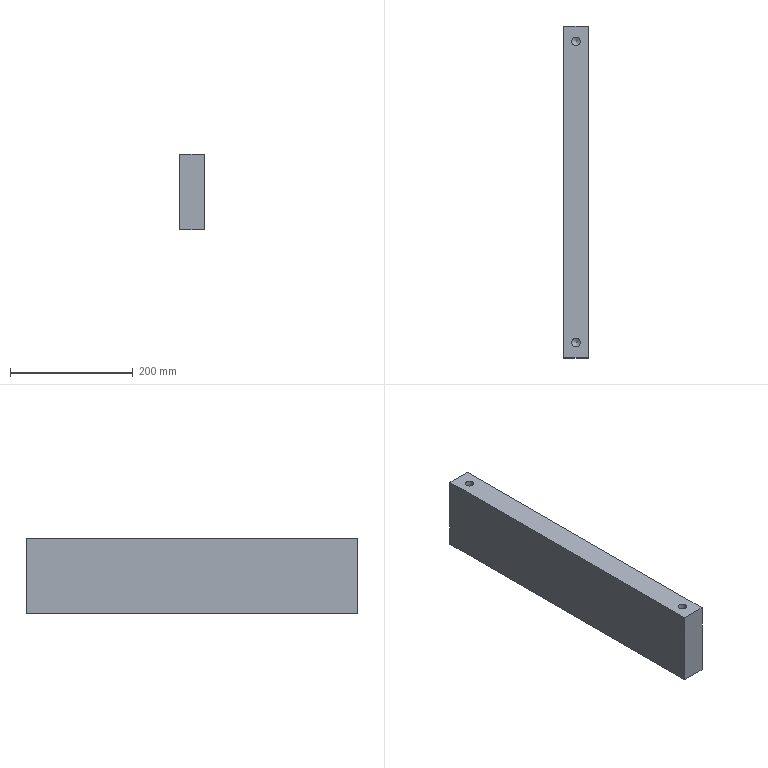Part | NX | features LIN_SOLID_COLOR 2 | 1 solid | 10 faces | box 40 x 540 x 123.5 mm | volume 2654870 mm3 | plane 6 | cylinder 2 | cone 2 | commonest cylinder face diameters 14 x2
STEP:
#1=CARTESIAN_POINT('',(266.,270.,-106.5));
#2=VERTEX_POINT('',#1);
#3=CARTESIAN_POINT('',(306.,270.,-106.5));
#4=VERTEX_POINT('',#3);
#5=CARTESIAN_POINT('',(306.,270.,-106.5));
#6=DIRECTION('',(1.,0.,0.));
#7=VECTOR('',#6,1000.);
#8=LINE('',#5,#7);
#9=EDGE_CURVE('',#2,#4,#8,.T.);
#10=ORIENTED_EDGE('',*,*,#9,.T.);
#11=CARTESIAN_POINT('',(306.,270.,-230.));
#12=VERTEX_POINT('',#11);
#13=CARTESIAN_POINT('',(306.,270.,-101.5));
#14=DIRECTION('',(0.,0.,1.));
#15=VECTOR('',#14,1000.);
#16=LINE('',#13,#15);
#17=EDGE_CURVE('',#12,#4,#16,.T.);
#18=ORIENTED_EDGE('',*,*,#17,.F.);
#19=CARTESIAN_POINT('',(266.,270.,-230.));
#20=VERTEX_POINT('',#19);
#21=CARTESIAN_POINT('',(446.,270.,-230.));
#22=DIRECTION('',(1.,0.,0.));
#23=VECTOR('',#22,1000.);
#24=LINE('',#21,#23);
#25=EDGE_CURVE('',#20,#12,#24,.T.);
#26=ORIENTED_EDGE('',*,*,#25,.F.);
#27=CARTESIAN_POINT('',(266.,270.,-101.5));
#28=DIRECTION('',(0.,0.,1.));
#29=VECTOR('',#28,1000.);
#30=LINE('',#27,#29);
#31=EDGE_CURVE('',#20,#2,#30,.T.);
#32=ORIENTED_EDGE('',*,*,#31,.T.);
#33=EDGE_LOOP('',(#10,#18,#26,#32));
#34=FACE_BOUND('',#33,.T.);
#35=CARTESIAN_POINT('',(306.,270.,-101.5));
#36=DIRECTION('',(0.,-1.,0.));
#37=DIRECTION('',(0.,0.,1.));
#38=AXIS2_PLACEMENT_3D('',#35,#36,#37);
#39=PLANE('',#38);
#40=ADVANCED_FACE('',(#34),#39,.F.);
#41=CARTESIAN_POINT('',(306.,-270.,-106.5));
#42=VERTEX_POINT('',#41);
#43=CARTESIAN_POINT('',(306.,0.,-106.5));
#44=DIRECTION('',(0.,1.,0.));
#45=VECTOR('',#44,1000.);
#46=LINE('',#43,#45);
#47=EDGE_CURVE('',#42,#4,#46,.T.);
#48=ORIENTED_EDGE('',*,*,#47,.F.);
#49=CARTESIAN_POINT('',(306.,-270.,-230.));
#50=VERTEX_POINT('',#49);
#51=CARTESIAN_POINT('',(306.,-270.,-101.5));
#52=DIRECTION('',(0.,0.,1.));
#53=VECTOR('',#52,1000.);
#54=LINE('',#51,#53);
#55=EDGE_CURVE('',#50,#42,#54,.T.);
#56=ORIENTED_EDGE('',*,*,#55,.F.);
#57=CARTESIAN_POINT('',(306.,0.,-230.));
#58=DIRECTION('',(0.,-1.,0.));
#59=VECTOR('',#58,1000.);
#60=LINE('',#57,#59);
#61=EDGE_CURVE('',#12,#50,#60,.T.);
#62=ORIENTED_EDGE('',*,*,#61,.F.);
#63=ORIENTED_EDGE('',*,*,#17,.T.);
#64=EDGE_LOOP('',(#48,#56,#62,#63));
#65=FACE_BOUND('',#64,.T.);
#66=CARTESIAN_POINT('',(306.,0.,-101.5));
#67=DIRECTION('',(-1.,0.,0.));
#68=DIRECTION('',(0.,0.,1.));
#69=AXIS2_PLACEMENT_3D('',#66,#67,#68);
#70=PLANE('',#69);
#71=ADVANCED_FACE('',(#65),#70,.F.);
#72=CARTESIAN_POINT('',(266.,-270.,-230.));
#73=VERTEX_POINT('',#72);
#74=CARTESIAN_POINT('',(266.,-270.,-106.5));
#75=VERTEX_POINT('',#74);
#76=CARTESIAN_POINT('',(266.,-270.,-101.5));
#77=DIRECTION('',(0.,0.,1.));
#78=VECTOR('',#77,1000.);
#79=LINE('',#76,#78);
#80=EDGE_CURVE('',#73,#75,#79,.T.);
#81=ORIENTED_EDGE('',*,*,#80,.T.);
#82=CARTESIAN_POINT('',(266.,0.,-106.5));
#83=DIRECTION('',(0.,1.,0.));
#84=VECTOR('',#83,1000.);
#85=LINE('',#82,#84);
#86=EDGE_CURVE('',#75,#2,#85,.T.);
#87=ORIENTED_EDGE('',*,*,#86,.T.);
#88=ORIENTED_EDGE('',*,*,#31,.F.);
#89=CARTESIAN_POINT('',(266.,0.,-230.));
#90=DIRECTION('',(0.,-1.,0.));
#91=VECTOR('',#90,1000.);
#92=LINE('',#89,#91);
#93=EDGE_CURVE('',#20,#73,#92,.T.);
#94=ORIENTED_EDGE('',*,*,#93,.T.);
#95=EDGE_LOOP('',(#81,#87,#88,#94));
#96=FACE_BOUND('',#95,.T.);
#97=CARTESIAN_POINT('',(266.,0.,-101.5));
#98=DIRECTION('',(-1.,0.,0.));
#99=DIRECTION('',(0.,0.,1.));
#100=AXIS2_PLACEMENT_3D('',#97,#98,#99);
#101=PLANE('',#100);
#102=ADVANCED_FACE('',(#96),#101,.T.);
#103=ORIENTED_EDGE('',*,*,#61,.T.);
#104=CARTESIAN_POINT('',(306.,-270.,-230.));
#105=DIRECTION('',(-1.,0.,0.));
#106=VECTOR('',#105,1000.);
#107=LINE('',#104,#106);
#108=EDGE_CURVE('',#73,#50,#107,.F.);
#109=ORIENTED_EDGE('',*,*,#108,.F.);
#110=ORIENTED_EDGE('',*,*,#93,.F.);
#111=ORIENTED_EDGE('',*,*,#25,.T.);
#112=EDGE_LOOP('',(#103,#109,#110,#111));
#113=FACE_BOUND('',#112,.T.);
#114=CARTESIAN_POINT('',(446.,0.,-230.));
#115=DIRECTION('',(0.,0.,1.));
#116=DIRECTION('',(1.,0.,0.));
#117=AXIS2_PLACEMENT_3D('',#114,#115,#116);
#118=PLANE('',#117);
#119=ADVANCED_FACE('',(#113),#118,.F.);
#120=CARTESIAN_POINT('',(279.,-245.,-106.5));
#121=VERTEX_POINT('',#120);
#122=CARTESIAN_POINT('',(286.,-245.,-106.5));
#123=DIRECTION('',(0.,0.,-1.));
#124=DIRECTION('',(-1.,0.,0.));
#125=AXIS2_PLACEMENT_3D('',#122,#123,#124);
#126=CIRCLE('',#125,7.);
#127=EDGE_CURVE('',#121,#121,#126,.T.);
#128=ORIENTED_EDGE('',*,*,#127,.T.);
#129=EDGE_LOOP('',(#128));
#130=FACE_BOUND('',#129,.T.);
#131=CARTESIAN_POINT('',(1036.,-270.,-106.5));
#132=DIRECTION('',(-1.,0.,0.));
#133=VECTOR('',#132,1000.);
#134=LINE('',#131,#133);
#135=EDGE_CURVE('',#75,#42,#134,.F.);
#136=ORIENTED_EDGE('',*,*,#135,.T.);
#137=ORIENTED_EDGE('',*,*,#47,.T.);
#138=ORIENTED_EDGE('',*,*,#9,.F.);
#139=ORIENTED_EDGE('',*,*,#86,.F.);
#140=EDGE_LOOP('',(#136,#137,#138,#139));
#141=FACE_BOUND('',#140,.T.);
#142=CARTESIAN_POINT('',(279.,245.,-106.5));
#143=VERTEX_POINT('',#142);
#144=CARTESIAN_POINT('',(286.,245.,-106.5));
#145=DIRECTION('',(0.,0.,-1.));
#146=DIRECTION('',(-1.,0.,0.));
#147=AXIS2_PLACEMENT_3D('',#144,#145,#146);
#148=CIRCLE('',#147,7.);
#149=EDGE_CURVE('',#143,#143,#148,.T.);
#150=ORIENTED_EDGE('',*,*,#149,.T.);
#151=EDGE_LOOP('',(#150));
#152=FACE_BOUND('',#151,.T.);
#153=CARTESIAN_POINT('',(1036.,0.,-106.5));
#154=DIRECTION('',(0.,0.,-1.));
#155=DIRECTION('',(-1.,0.,0.));
#156=AXIS2_PLACEMENT_3D('',#153,#154,#155);
#157=PLANE('',#156);
#158=ADVANCED_FACE('',(#130,#141,#152),#157,.F.);
#159=ORIENTED_EDGE('',*,*,#108,.T.);
#160=ORIENTED_EDGE('',*,*,#55,.T.);
#161=ORIENTED_EDGE('',*,*,#135,.F.);
#162=ORIENTED_EDGE('',*,*,#80,.F.);
#163=EDGE_LOOP('',(#159,#160,#161,#162));
#164=FACE_BOUND('',#163,.T.);
#165=CARTESIAN_POINT('',(306.,-270.,-101.5));
#166=DIRECTION('',(0.,-1.,0.));
#167=DIRECTION('',(0.,0.,1.));
#168=AXIS2_PLACEMENT_3D('',#165,#166,#167);
#169=PLANE('',#168);
#170=ADVANCED_FACE('',(#164),#169,.T.);
#171=CARTESIAN_POINT('',(293.,-245.,-146.5));
#172=VERTEX_POINT('',#171);
#173=CARTESIAN_POINT('',(286.,-245.,-146.5));
#174=DIRECTION('',(0.,0.,1.));
#175=DIRECTION('',(1.,0.,0.));
#176=AXIS2_PLACEMENT_3D('',#173,#174,#175);
#177=CIRCLE('',#176,7.);
#178=EDGE_CURVE('',#172,#172,#177,.T.);
#179=ORIENTED_EDGE('',*,*,#178,.F.);
#180=EDGE_LOOP('',(#179));
#181=FACE_BOUND('',#180,.T.);
#182=ORIENTED_EDGE('',*,*,#127,.F.);
#183=EDGE_LOOP('',(#182));
#184=FACE_BOUND('',#183,.T.);
#185=CARTESIAN_POINT('',(286.,-245.,-106.4));
#186=DIRECTION('',(0.,0.,-1.));
#187=DIRECTION('',(1.,0.,0.));
#188=AXIS2_PLACEMENT_3D('',#185,#186,#187);
#189=CYLINDRICAL_SURFACE('',#188,7.);
#190=ADVANCED_FACE('',(#181,#184),#189,.F.);
#191=ORIENTED_EDGE('',*,*,#178,.T.);
#192=EDGE_LOOP('',(#191));
#193=FACE_BOUND('',#192,.T.);
#194=CARTESIAN_POINT('',(286.,-245.,-150.541));
#195=VERTEX_POINT('',#194);
#196=VERTEX_LOOP('',#195);
#197=FACE_BOUND('',#196,.T.);
#198=CARTESIAN_POINT('',(286.,-245.,-150.541));
#199=DIRECTION('',(0.,0.,1.));
#200=DIRECTION('',(1.,0.,0.));
#201=AXIS2_PLACEMENT_3D('',#198,#199,#200);
#202=CONICAL_SURFACE('',#201,0.,1.047);
#203=ADVANCED_FACE('',(#193,#197),#202,.F.);
#204=CARTESIAN_POINT('',(293.,245.,-146.5));
#205=VERTEX_POINT('',#204);
#206=CARTESIAN_POINT('',(286.,245.,-146.5));
#207=DIRECTION('',(0.,0.,1.));
#208=DIRECTION('',(1.,0.,0.));
#209=AXIS2_PLACEMENT_3D('',#206,#207,#208);
#210=CIRCLE('',#209,7.);
#211=EDGE_CURVE('',#205,#205,#210,.T.);
#212=ORIENTED_EDGE('',*,*,#211,.F.);
#213=EDGE_LOOP('',(#212));
#214=FACE_BOUND('',#213,.T.);
#215=ORIENTED_EDGE('',*,*,#149,.F.);
#216=EDGE_LOOP('',(#215));
#217=FACE_BOUND('',#216,.T.);
#218=CARTESIAN_POINT('',(286.,245.,-106.4));
#219=DIRECTION('',(0.,0.,-1.));
#220=DIRECTION('',(1.,0.,0.));
#221=AXIS2_PLACEMENT_3D('',#218,#219,#220);
#222=CYLINDRICAL_SURFACE('',#221,7.);
#223=ADVANCED_FACE('',(#214,#217),#222,.F.);
#224=ORIENTED_EDGE('',*,*,#211,.T.);
#225=EDGE_LOOP('',(#224));
#226=FACE_BOUND('',#225,.T.);
#227=CARTESIAN_POINT('',(286.,245.,-150.541));
#228=VERTEX_POINT('',#227);
#229=VERTEX_LOOP('',#228);
#230=FACE_BOUND('',#229,.T.);
#231=CARTESIAN_POINT('',(286.,245.,-150.541));
#232=DIRECTION('',(0.,0.,1.));
#233=DIRECTION('',(1.,0.,0.));
#234=AXIS2_PLACEMENT_3D('',#231,#232,#233);
#235=CONICAL_SURFACE('',#234,0.,1.047);
#236=ADVANCED_FACE('',(#226,#230),#235,.F.);
#237=CLOSED_SHELL('',(#40,#71,#102,#119,#158,#170,#190,#203,#223,#236));
#238=MANIFOLD_SOLID_BREP('',#237);
#239=(LENGTH_UNIT()NAMED_UNIT(*)SI_UNIT(.MILLI.,.METRE.));
#240=UNCERTAINTY_MEASURE_WITH_UNIT(LENGTH_MEASURE(0.00001),#239,'','');
#241=(NAMED_UNIT(*)PLANE_ANGLE_UNIT()SI_UNIT($,.RADIAN.));
#242=(NAMED_UNIT(*)SI_UNIT($,.STERADIAN.)SOLID_ANGLE_UNIT());
#243=(GEOMETRIC_REPRESENTATION_CONTEXT(3)GLOBAL_UNCERTAINTY_ASSIGNED_CONTEXT((#240))GLOBAL_UNIT_ASSIGNED_CONTEXT((#239,#241,#242))REPRESENTATION_CONTEXT('',''));
#244=ADVANCED_BREP_SHAPE_REPRESENTATION('',(#238),#243);